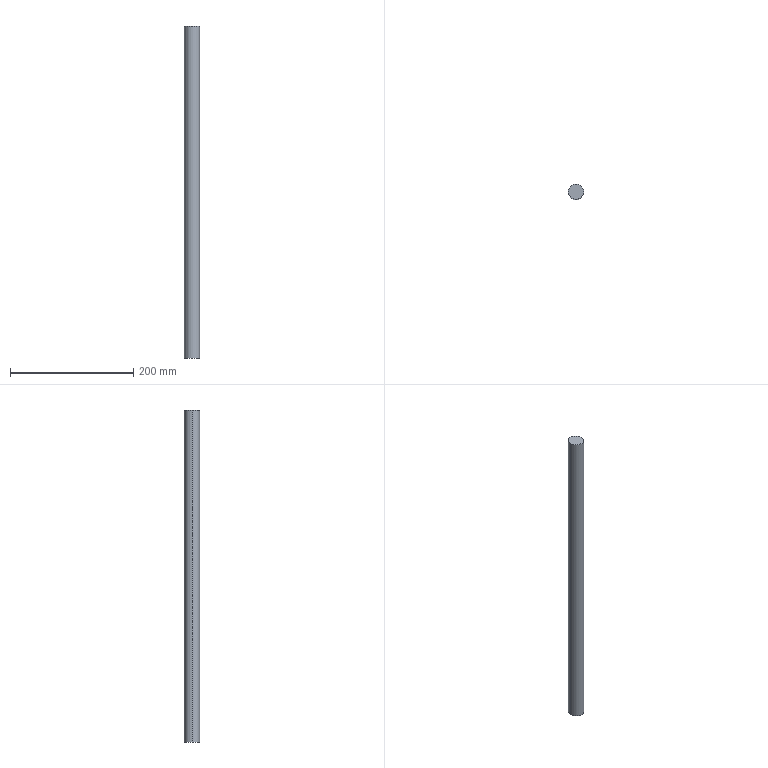Part | STEP file | Shaft dia 25 for small 21V11 | 1 solid | 4 faces | box 25 x 25 x 539.4 mm | volume 264777 mm3 | cylinder 2 | plane 2 | commonest cylinder face diameters 25 x2
STEP:
#1=CARTESIAN_POINT('',(0.,0.,0.));
#2=DIRECTION('',(0.,0.,1.));
#3=DIRECTION('',(1.,0.,0.));
#4=AXIS2_PLACEMENT_3D('',#1,#2,#3);
#5=CARTESIAN_POINT('',(12.5,0.,539.4));
#6=VERTEX_POINT('',#5);
#7=CARTESIAN_POINT('',(-12.5,0.,539.4));
#8=VERTEX_POINT('',#7);
#9=CARTESIAN_POINT('',(0.,0.,539.4));
#10=DIRECTION('',(0.,0.,1.));
#11=DIRECTION('',(1.,0.,0.));
#12=AXIS2_PLACEMENT_3D('',#9,#10,#11);
#13=CIRCLE('',#12,12.5);
#14=CARTESIAN_POINT('',(0.,0.,539.4));
#15=DIRECTION('',(0.,0.,-1.));
#16=DIRECTION('',(-1.,0.,0.));
#17=AXIS2_PLACEMENT_3D('',#14,#15,#16);
#18=CYLINDRICAL_SURFACE('',#17,12.5);
#19=CARTESIAN_POINT('',(3.142,0.));
#20=DIRECTION('',(-1.,0.));
#21=VECTOR('',#20,1.);
#22=LINE('',#19,#21);
#23=(GEOMETRIC_REPRESENTATION_CONTEXT(2)PARAMETRIC_REPRESENTATION_CONTEXT()REPRESENTATION_CONTEXT('',''));
#24=DEFINITIONAL_REPRESENTATION('',(#22),#23);
#25=PCURVE('',#18,#24);
#26=CARTESIAN_POINT('',(0.,0.,539.4));
#27=DIRECTION('',(0.,0.,1.));
#28=DIRECTION('',(1.,0.,0.));
#29=AXIS2_PLACEMENT_3D('',#26,#27,#28);
#30=PLANE('',#29);
#31=CARTESIAN_POINT('',(0.,0.));
#32=DIRECTION('',(1.,0.));
#33=AXIS2_PLACEMENT_2D('',#31,#32);
#34=CIRCLE('',#33,12.5);
#35=(GEOMETRIC_REPRESENTATION_CONTEXT(2)PARAMETRIC_REPRESENTATION_CONTEXT()REPRESENTATION_CONTEXT('',''));
#36=DEFINITIONAL_REPRESENTATION('',(#34),#35);
#37=PCURVE('',#30,#36);
#38=SURFACE_CURVE('',#13,(#25,#37),.PCURVE_S1.);
#39=EDGE_CURVE('',#6,#8,#38,.T.);
#40=ORIENTED_EDGE('',*,*,#39,.F.);
#41=CARTESIAN_POINT('',(12.5,0.,0.));
#42=VERTEX_POINT('',#41);
#43=CARTESIAN_POINT('',(12.5,0.,539.4));
#44=DIRECTION('',(0.,0.,-1.));
#45=VECTOR('',#44,1.);
#46=LINE('',#43,#45);
#47=CARTESIAN_POINT('',(3.142,0.));
#48=DIRECTION('',(0.,1.));
#49=VECTOR('',#48,1.);
#50=LINE('',#47,#49);
#51=(GEOMETRIC_REPRESENTATION_CONTEXT(2)PARAMETRIC_REPRESENTATION_CONTEXT()REPRESENTATION_CONTEXT('',''));
#52=DEFINITIONAL_REPRESENTATION('',(#50),#51);
#53=PCURVE('',#18,#52);
#54=CARTESIAN_POINT('',(0.,0.,539.4));
#55=DIRECTION('',(0.,0.,-1.));
#56=DIRECTION('',(-1.,0.,0.));
#57=AXIS2_PLACEMENT_3D('',#54,#55,#56);
#58=CYLINDRICAL_SURFACE('',#57,12.5);
#59=CARTESIAN_POINT('',(3.142,0.));
#60=DIRECTION('',(0.,1.));
#61=VECTOR('',#60,1.);
#62=LINE('',#59,#61);
#63=(GEOMETRIC_REPRESENTATION_CONTEXT(2)PARAMETRIC_REPRESENTATION_CONTEXT()REPRESENTATION_CONTEXT('',''));
#64=DEFINITIONAL_REPRESENTATION('',(#62),#63);
#65=PCURVE('',#58,#64);
#66=SURFACE_CURVE('',#46,(#53,#65),.PCURVE_S1.);
#67=EDGE_CURVE('',#6,#42,#66,.T.);
#68=ORIENTED_EDGE('',*,*,#67,.T.);
#69=CARTESIAN_POINT('',(-12.5,0.,0.));
#70=VERTEX_POINT('',#69);
#71=CARTESIAN_POINT('',(0.,0.,0.));
#72=DIRECTION('',(0.,0.,1.));
#73=DIRECTION('',(1.,0.,0.));
#74=AXIS2_PLACEMENT_3D('',#71,#72,#73);
#75=CIRCLE('',#74,12.5);
#76=CARTESIAN_POINT('',(3.142,539.4));
#77=DIRECTION('',(-1.,0.));
#78=VECTOR('',#77,1.);
#79=LINE('',#76,#78);
#80=(GEOMETRIC_REPRESENTATION_CONTEXT(2)PARAMETRIC_REPRESENTATION_CONTEXT()REPRESENTATION_CONTEXT('',''));
#81=DEFINITIONAL_REPRESENTATION('',(#79),#80);
#82=PCURVE('',#18,#81);
#83=CARTESIAN_POINT('',(0.,0.,0.));
#84=DIRECTION('',(0.,0.,1.));
#85=DIRECTION('',(1.,0.,0.));
#86=AXIS2_PLACEMENT_3D('',#83,#84,#85);
#87=PLANE('',#86);
#88=CARTESIAN_POINT('',(0.,0.));
#89=DIRECTION('',(1.,0.));
#90=AXIS2_PLACEMENT_2D('',#88,#89);
#91=CIRCLE('',#90,12.5);
#92=(GEOMETRIC_REPRESENTATION_CONTEXT(2)PARAMETRIC_REPRESENTATION_CONTEXT()REPRESENTATION_CONTEXT('',''));
#93=DEFINITIONAL_REPRESENTATION('',(#91),#92);
#94=PCURVE('',#87,#93);
#95=SURFACE_CURVE('',#75,(#82,#94),.PCURVE_S1.);
#96=EDGE_CURVE('',#42,#70,#95,.T.);
#97=ORIENTED_EDGE('',*,*,#96,.T.);
#98=CARTESIAN_POINT('',(-12.5,0.,539.4));
#99=DIRECTION('',(0.,0.,-1.));
#100=VECTOR('',#99,1.);
#101=LINE('',#98,#100);
#102=CARTESIAN_POINT('',(0.,0.));
#103=DIRECTION('',(0.,1.));
#104=VECTOR('',#103,1.);
#105=LINE('',#102,#104);
#106=(GEOMETRIC_REPRESENTATION_CONTEXT(2)PARAMETRIC_REPRESENTATION_CONTEXT()REPRESENTATION_CONTEXT('',''));
#107=DEFINITIONAL_REPRESENTATION('',(#105),#106);
#108=PCURVE('',#18,#107);
#109=CARTESIAN_POINT('',(6.283,0.));
#110=DIRECTION('',(0.,1.));
#111=VECTOR('',#110,1.);
#112=LINE('',#109,#111);
#113=(GEOMETRIC_REPRESENTATION_CONTEXT(2)PARAMETRIC_REPRESENTATION_CONTEXT()REPRESENTATION_CONTEXT('',''));
#114=DEFINITIONAL_REPRESENTATION('',(#112),#113);
#115=PCURVE('',#58,#114);
#116=SURFACE_CURVE('',#101,(#108,#115),.PCURVE_S1.);
#117=EDGE_CURVE('',#8,#70,#116,.T.);
#118=ORIENTED_EDGE('',*,*,#117,.F.);
#119=EDGE_LOOP('',(#40,#68,#97,#118));
#120=FACE_BOUND('',#119,.T.);
#121=ADVANCED_FACE('',(#120),#18,.T.);
#122=ORIENTED_EDGE('',*,*,#67,.F.);
#123=CARTESIAN_POINT('',(0.,0.,539.4));
#124=DIRECTION('',(0.,0.,1.));
#125=DIRECTION('',(1.,0.,0.));
#126=AXIS2_PLACEMENT_3D('',#123,#124,#125);
#127=CIRCLE('',#126,12.5);
#128=CARTESIAN_POINT('',(9.425,0.));
#129=DIRECTION('',(-1.,0.));
#130=VECTOR('',#129,1.);
#131=LINE('',#128,#130);
#132=(GEOMETRIC_REPRESENTATION_CONTEXT(2)PARAMETRIC_REPRESENTATION_CONTEXT()REPRESENTATION_CONTEXT('',''));
#133=DEFINITIONAL_REPRESENTATION('',(#131),#132);
#134=PCURVE('',#58,#133);
#135=CARTESIAN_POINT('',(0.,0.));
#136=DIRECTION('',(1.,0.));
#137=AXIS2_PLACEMENT_2D('',#135,#136);
#138=CIRCLE('',#137,12.5);
#139=(GEOMETRIC_REPRESENTATION_CONTEXT(2)PARAMETRIC_REPRESENTATION_CONTEXT()REPRESENTATION_CONTEXT('',''));
#140=DEFINITIONAL_REPRESENTATION('',(#138),#139);
#141=PCURVE('',#30,#140);
#142=SURFACE_CURVE('',#127,(#134,#141),.PCURVE_S1.);
#143=EDGE_CURVE('',#8,#6,#142,.T.);
#144=ORIENTED_EDGE('',*,*,#143,.F.);
#145=ORIENTED_EDGE('',*,*,#117,.T.);
#146=CARTESIAN_POINT('',(0.,0.,0.));
#147=DIRECTION('',(0.,0.,1.));
#148=DIRECTION('',(1.,0.,0.));
#149=AXIS2_PLACEMENT_3D('',#146,#147,#148);
#150=CIRCLE('',#149,12.5);
#151=CARTESIAN_POINT('',(9.425,539.4));
#152=DIRECTION('',(-1.,0.));
#153=VECTOR('',#152,1.);
#154=LINE('',#151,#153);
#155=(GEOMETRIC_REPRESENTATION_CONTEXT(2)PARAMETRIC_REPRESENTATION_CONTEXT()REPRESENTATION_CONTEXT('',''));
#156=DEFINITIONAL_REPRESENTATION('',(#154),#155);
#157=PCURVE('',#58,#156);
#158=CARTESIAN_POINT('',(0.,0.));
#159=DIRECTION('',(1.,0.));
#160=AXIS2_PLACEMENT_2D('',#158,#159);
#161=CIRCLE('',#160,12.5);
#162=(GEOMETRIC_REPRESENTATION_CONTEXT(2)PARAMETRIC_REPRESENTATION_CONTEXT()REPRESENTATION_CONTEXT('',''));
#163=DEFINITIONAL_REPRESENTATION('',(#161),#162);
#164=PCURVE('',#87,#163);
#165=SURFACE_CURVE('',#150,(#157,#164),.PCURVE_S1.);
#166=EDGE_CURVE('',#70,#42,#165,.T.);
#167=ORIENTED_EDGE('',*,*,#166,.T.);
#168=EDGE_LOOP('',(#122,#144,#145,#167));
#169=FACE_BOUND('',#168,.T.);
#170=ADVANCED_FACE('',(#169),#58,.T.);
#171=ORIENTED_EDGE('',*,*,#143,.T.);
#172=ORIENTED_EDGE('',*,*,#39,.T.);
#173=EDGE_LOOP('',(#171,#172));
#174=FACE_BOUND('',#173,.T.);
#175=ADVANCED_FACE('',(#174),#30,.T.);
#176=ORIENTED_EDGE('',*,*,#166,.F.);
#177=ORIENTED_EDGE('',*,*,#96,.F.);
#178=EDGE_LOOP('',(#176,#177));
#179=FACE_BOUND('',#178,.T.);
#180=ADVANCED_FACE('',(#179),#87,.F.);
#181=CLOSED_SHELL('',(#121,#170,#175,#180));
#182=MANIFOLD_SOLID_BREP('',#181);
#183=(LENGTH_UNIT()NAMED_UNIT(*)SI_UNIT(.MILLI.,.METRE.));
#184=UNCERTAINTY_MEASURE_WITH_UNIT(LENGTH_MEASURE(0.0000001),#183,'','');
#185=(NAMED_UNIT(*)PLANE_ANGLE_UNIT()SI_UNIT($,.RADIAN.));
#186=(NAMED_UNIT(*)SI_UNIT($,.STERADIAN.)SOLID_ANGLE_UNIT());
#187=(GEOMETRIC_REPRESENTATION_CONTEXT(3)GLOBAL_UNCERTAINTY_ASSIGNED_CONTEXT((#184))GLOBAL_UNIT_ASSIGNED_CONTEXT((#183,#185,#186))REPRESENTATION_CONTEXT('',''));
#188=ADVANCED_BREP_SHAPE_REPRESENTATION('',(#4,#182),#187);